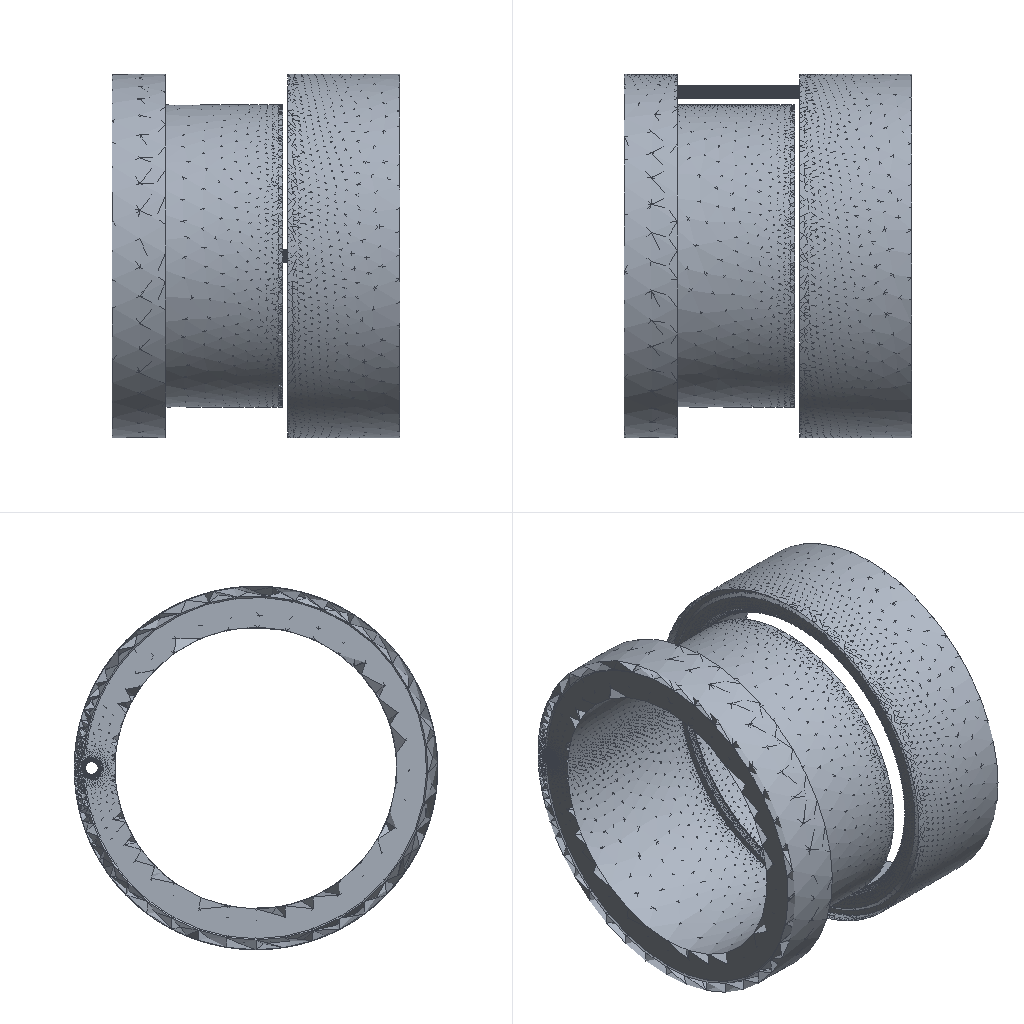Simulation study | ansys fluent
Set-up summary:
category,name,step,type,value,unit,region
solver,ansys_fluent,,Fluent 26.1.0
units,SI m-kg-s (Fluent internal),,stated,boundary values in the units shown in brackets; results in listed units
analysis,deck.cas,,cfd steady,"dimension=3D; solver=3d, dp, pbns, sstkw (3d, double precision, pressure-based, SST k-omega); source_case=.cas.h5"
model,Space,deck.cas,,3D
model,Time,deck.cas,,Steady
model,Viscous,deck.cas,,SST k-omega turbulence model
model,Heat Transfer,deck.cas,,Disabled
model,Multiphase,deck.cas,,Disabled
mesh,nodes,,,206228
mesh,elements,,,847816
mesh,faces,,,1824283
cell_zone,part_1,deck.cas,fluid,material=gasoil-liquid,,zone 3
material,gasoil-liquid (fluid),,Density,830,kg/m^3
material,gasoil-liquid (fluid),,Viscosity,0.01252,kg/(m s)
material,air (fluid),,Density,1.225,kg/m^3
material,air (fluid),,Viscosity,1.7894e-05,kg/(m s)
material,aluminum (solid),,Density,2719,kg/m^3
bc,int,deck.cas,velocity-inlet,Velocity Magnitude [m/s]=0.2,,zone 6
bc,wall-part_1,deck.cas,wall,Wall Motion=Stationary Wall; Shear Boundary Condition=No Slip; Wall Surface Roughness=Standard,,zone 1
bc,out,deck.cas,pressure-outlet,Gauge Pressure [Pa]=30000000,,zone 7
Results summary:
result,mass flow rate int,deck.cas,,0.1306,kg/s
result,mass flow rate out,deck.cas,,-0.1181,kg/s
result,mass flow rate wall-part_1,deck.cas,,-0,kg/s
result,mass flow rate Net,deck.cas,,0.01257,kg/s
result,wall force total wall-part_1,deck.cas,,"(1.0113e+06, -0.1212, 0.06886)",N
result,wall force pressure wall-part_1,deck.cas,,"(1.01077e+06, -0.3679, -0.5492)",N
result,wall force viscous wall-part_1,deck.cas,,"(527.523, 0.2467, 0.6181)",N
result,wall force total Net,deck.cas,,"(1.0113e+06, -0.1212, 0.06886)",N
result,wall force pressure Net,deck.cas,,"(1.01077e+06, -0.3679, -0.5492)",N
result,wall force viscous Net,deck.cas,,"(527.523, 0.2467, 0.6181)",N